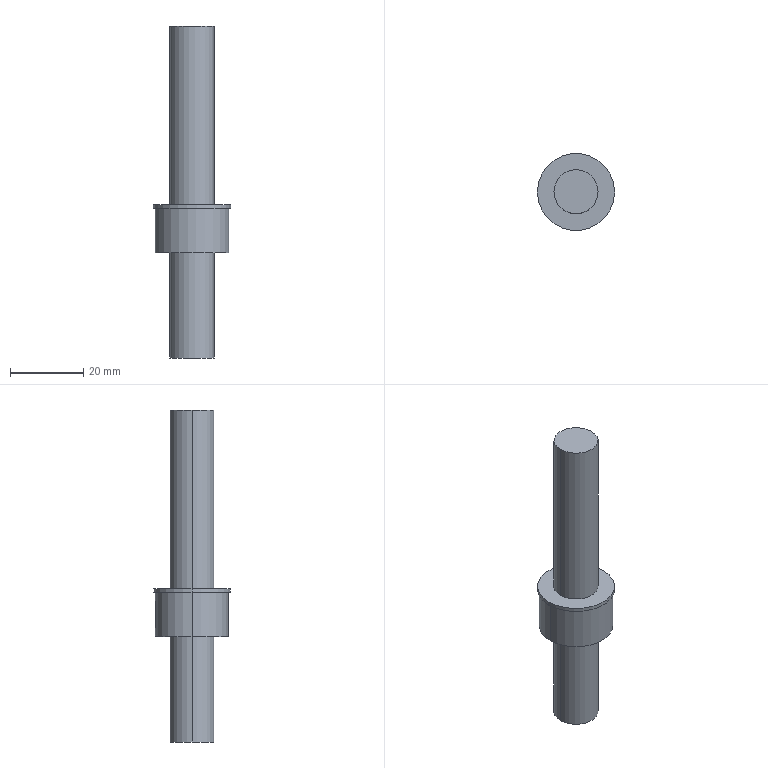Part | SolidWorks | features ICE 4, Extrusion 1 | 1 solid | 19 faces | box 21 x 21 x 90.35 mm | volume 12865 mm3 | cylinder 11 | plane 8 | commonest cylinder face diameters 12 x4 3 x3 20 x2 21 x2
STEP:
#1=CARTESIAN_POINT('',(0.,9.1,38.75));
#2=VERTEX_POINT('',#1);
#3=CARTESIAN_POINT('',(1.5,9.1,37.25));
#4=VERTEX_POINT('',#3);
#5=CARTESIAN_POINT('',(0.,9.1,37.25));
#6=DIRECTION('',(0.,1.,0.));
#7=DIRECTION('',(0.,0.,1.));
#8=AXIS2_PLACEMENT_3D('',#5,#6,#7);
#9=CIRCLE('',#8,1.5);
#10=EDGE_CURVE('',#2,#4,#9,.T.);
#11=ORIENTED_EDGE('',*,*,#10,.F.);
#12=CARTESIAN_POINT('',(0.,10.,38.75));
#13=VERTEX_POINT('',#12);
#14=CARTESIAN_POINT('',(0.,9.1,38.75));
#15=DIRECTION('',(0.,1.,0.));
#16=VECTOR('',#15,1000.);
#17=LINE('',#14,#16);
#18=EDGE_CURVE('',#2,#13,#17,.T.);
#19=ORIENTED_EDGE('',*,*,#18,.T.);
#20=CARTESIAN_POINT('',(1.5,9.887,37.25));
#21=VERTEX_POINT('',#20);
#22=CARTESIAN_POINT('',(1.5,9.887,37.25));
#23=CARTESIAN_POINT('',(1.5,9.887,37.349));
#24=CARTESIAN_POINT('',(1.49,9.888,37.447));
#25=CARTESIAN_POINT('',(1.452,9.894,37.639));
#26=CARTESIAN_POINT('',(1.423,9.898,37.734));
#27=CARTESIAN_POINT('',(1.348,9.909,37.916));
#28=CARTESIAN_POINT('',(1.302,9.915,38.002));
#29=CARTESIAN_POINT('',(1.193,9.929,38.165));
#30=CARTESIAN_POINT('',(1.129,9.936,38.242));
#31=CARTESIAN_POINT('',(0.922,9.958,38.449));
#32=CARTESIAN_POINT('',(0.7548,9.973,38.561));
#33=CARTESIAN_POINT('',(0.3937,9.994,38.711));
#34=CARTESIAN_POINT('',(0.196,10.,38.75));
#35=CARTESIAN_POINT('',(0.,10.,38.75));
#36=B_SPLINE_CURVE_WITH_KNOTS('',3,(#22,#23,#24,#25,#26,#27,#28,#29,#30,#31,#32,#33,#34,#35),.UNSPECIFIED.,.F.,.F.,(4,2,2,2,2,2,4),(0.,0.0002936,0.0005872,0.0008808,0.001174,0.001762,0.002349),.UNSPECIFIED.);
#37=EDGE_CURVE('',#21,#13,#36,.T.);
#38=ORIENTED_EDGE('',*,*,#37,.F.);
#39=CARTESIAN_POINT('',(1.5,9.1,37.25));
#40=DIRECTION('',(0.,1.,0.));
#41=VECTOR('',#40,1000.);
#42=LINE('',#39,#41);
#43=EDGE_CURVE('',#4,#21,#42,.T.);
#44=ORIENTED_EDGE('',*,*,#43,.F.);
#45=EDGE_LOOP('',(#11,#19,#38,#44));
#46=FACE_OUTER_BOUND('',#45,.T.);
#47=CARTESIAN_POINT('',(0.,9.1,37.25));
#48=DIRECTION('',(0.,1.,0.));
#49=DIRECTION('',(0.,0.,1.));
#50=AXIS2_PLACEMENT_3D('',#47,#48,#49);
#51=CYLINDRICAL_SURFACE('',#50,1.5);
#52=ADVANCED_FACE('',(#46),#51,.F.);
#53=CARTESIAN_POINT('',(6.,0.,90.35));
#54=VERTEX_POINT('',#53);
#55=CARTESIAN_POINT('',(-6.,0.,90.35));
#56=VERTEX_POINT('',#55);
#57=CARTESIAN_POINT('',(0.,0.,90.35));
#58=DIRECTION('',(0.,0.,1.));
#59=DIRECTION('',(1.,0.,0.));
#60=AXIS2_PLACEMENT_3D('',#57,#58,#59);
#61=CIRCLE('',#60,6.);
#62=EDGE_CURVE('',#54,#56,#61,.T.);
#63=ORIENTED_EDGE('',*,*,#62,.F.);
#64=CARTESIAN_POINT('',(6.,0.,41.75));
#65=VERTEX_POINT('',#64);
#66=CARTESIAN_POINT('',(6.,0.,90.35));
#67=DIRECTION('',(0.,0.,-1.));
#68=VECTOR('',#67,1000.);
#69=LINE('',#66,#68);
#70=EDGE_CURVE('',#54,#65,#69,.T.);
#71=ORIENTED_EDGE('',*,*,#70,.T.);
#72=CARTESIAN_POINT('',(-6.,0.,41.75));
#73=VERTEX_POINT('',#72);
#74=CARTESIAN_POINT('',(0.,0.,41.75));
#75=DIRECTION('',(0.,0.,1.));
#76=DIRECTION('',(1.,0.,0.));
#77=AXIS2_PLACEMENT_3D('',#74,#75,#76);
#78=CIRCLE('',#77,6.);
#79=EDGE_CURVE('',#65,#73,#78,.T.);
#80=ORIENTED_EDGE('',*,*,#79,.T.);
#81=CARTESIAN_POINT('',(-6.,0.,90.35));
#82=DIRECTION('',(0.,0.,-1.));
#83=VECTOR('',#82,1000.);
#84=LINE('',#81,#83);
#85=EDGE_CURVE('',#56,#73,#84,.T.);
#86=ORIENTED_EDGE('',*,*,#85,.F.);
#87=EDGE_LOOP('',(#63,#71,#80,#86));
#88=FACE_OUTER_BOUND('',#87,.T.);
#89=CARTESIAN_POINT('',(0.,0.,90.35));
#90=DIRECTION('',(0.,0.,-1.));
#91=DIRECTION('',(-1.,0.,0.));
#92=AXIS2_PLACEMENT_3D('',#89,#90,#91);
#93=CYLINDRICAL_SURFACE('',#92,6.);
#94=ADVANCED_FACE('',(#88),#93,.T.);
#95=CARTESIAN_POINT('',(10.5,0.,41.75));
#96=VERTEX_POINT('',#95);
#97=CARTESIAN_POINT('',(-10.5,0.,41.75));
#98=VERTEX_POINT('',#97);
#99=CARTESIAN_POINT('',(0.,0.,41.75));
#100=DIRECTION('',(0.,0.,1.));
#101=DIRECTION('',(1.,0.,0.));
#102=AXIS2_PLACEMENT_3D('',#99,#100,#101);
#103=CIRCLE('',#102,10.5);
#104=EDGE_CURVE('',#96,#98,#103,.T.);
#105=ORIENTED_EDGE('',*,*,#104,.F.);
#106=CARTESIAN_POINT('',(10.5,0.,40.75));
#107=VERTEX_POINT('',#106);
#108=CARTESIAN_POINT('',(10.5,0.,41.75));
#109=DIRECTION('',(0.,0.,-1.));
#110=VECTOR('',#109,1000.);
#111=LINE('',#108,#110);
#112=EDGE_CURVE('',#96,#107,#111,.T.);
#113=ORIENTED_EDGE('',*,*,#112,.T.);
#114=CARTESIAN_POINT('',(-10.5,0.,40.75));
#115=VERTEX_POINT('',#114);
#116=CARTESIAN_POINT('',(0.,0.,40.75));
#117=DIRECTION('',(0.,0.,1.));
#118=DIRECTION('',(1.,0.,0.));
#119=AXIS2_PLACEMENT_3D('',#116,#117,#118);
#120=CIRCLE('',#119,10.5);
#121=EDGE_CURVE('',#107,#115,#120,.T.);
#122=ORIENTED_EDGE('',*,*,#121,.T.);
#123=CARTESIAN_POINT('',(-10.5,0.,41.75));
#124=DIRECTION('',(0.,0.,-1.));
#125=VECTOR('',#124,1000.);
#126=LINE('',#123,#125);
#127=EDGE_CURVE('',#98,#115,#126,.T.);
#128=ORIENTED_EDGE('',*,*,#127,.F.);
#129=EDGE_LOOP('',(#105,#113,#122,#128));
#130=FACE_OUTER_BOUND('',#129,.T.);
#131=CARTESIAN_POINT('',(0.,0.,41.75));
#132=DIRECTION('',(0.,0.,-1.));
#133=DIRECTION('',(-1.,0.,0.));
#134=AXIS2_PLACEMENT_3D('',#131,#132,#133);
#135=CYLINDRICAL_SURFACE('',#134,10.5);
#136=ADVANCED_FACE('',(#130),#135,.T.);
#137=CARTESIAN_POINT('',(-1.5,9.887,37.25));
#138=VERTEX_POINT('',#137);
#139=CARTESIAN_POINT('',(-1.5,9.887,32.25));
#140=VERTEX_POINT('',#139);
#141=CARTESIAN_POINT('',(-1.5,9.887,40.75));
#142=DIRECTION('',(0.,0.,-1.));
#143=VECTOR('',#142,1000.);
#144=LINE('',#141,#143);
#145=EDGE_CURVE('',#138,#140,#144,.T.);
#146=ORIENTED_EDGE('',*,*,#145,.T.);
#147=CARTESIAN_POINT('',(1.5,9.887,32.25));
#148=VERTEX_POINT('',#147);
#149=CARTESIAN_POINT('',(-1.5,9.887,32.25));
#150=CARTESIAN_POINT('',(-1.5,9.887,32.151));
#151=CARTESIAN_POINT('',(-1.49,9.888,32.053));
#152=CARTESIAN_POINT('',(-1.452,9.894,31.861));
#153=CARTESIAN_POINT('',(-1.423,9.898,31.766));
#154=CARTESIAN_POINT('',(-1.348,9.909,31.584));
#155=CARTESIAN_POINT('',(-1.302,9.915,31.498));
#156=CARTESIAN_POINT('',(-1.193,9.929,31.335));
#157=CARTESIAN_POINT('',(-1.13,9.936,31.258));
#158=CARTESIAN_POINT('',(-0.9225,9.958,31.051));
#159=CARTESIAN_POINT('',(-0.7554,9.973,30.939));
#160=CARTESIAN_POINT('',(-0.3946,9.994,30.79));
#161=CARTESIAN_POINT('',(-0.1971,10.,30.75));
#162=CARTESIAN_POINT('',(0.09684,10.,30.75));
#163=CARTESIAN_POINT('',(0.1964,9.999,30.76));
#164=CARTESIAN_POINT('',(0.3888,9.993,30.798));
#165=CARTESIAN_POINT('',(0.4824,9.989,30.826));
#166=CARTESIAN_POINT('',(0.7551,9.973,30.939));
#167=CARTESIAN_POINT('',(0.9202,9.959,31.049));
#168=CARTESIAN_POINT('',(1.13,9.936,31.259));
#169=CARTESIAN_POINT('',(1.192,9.929,31.334));
#170=CARTESIAN_POINT('',(1.301,9.915,31.496));
#171=CARTESIAN_POINT('',(1.348,9.909,31.584));
#172=CARTESIAN_POINT('',(1.461,9.893,31.856));
#173=CARTESIAN_POINT('',(1.5,9.887,32.052));
#174=CARTESIAN_POINT('',(1.5,9.887,32.25));
#175=B_SPLINE_CURVE_WITH_KNOTS('',3,(#149,#150,#151,#152,#153,#154,#155,#156,#157,#158,#159,#160,#161,#162,#163,#164,#165,#166,#167,#168,#169,#170,#171,#172,#173,#174),.UNSPECIFIED.,.F.,.F.,(4,2,2,2,2,2,2,2,2,2,2,2,4),(0.,0.0002934,0.0005869,0.0008803,0.001174,0.001761,0.002348,0.002641,0.002934,0.003521,0.003815,0.004108,0.004695),.UNSPECIFIED.);
#176=EDGE_CURVE('',#140,#148,#175,.T.);
#177=ORIENTED_EDGE('',*,*,#176,.T.);
#178=CARTESIAN_POINT('',(1.5,9.887,40.75));
#179=DIRECTION('',(0.,0.,1.));
#180=VECTOR('',#179,1000.);
#181=LINE('',#178,#180);
#182=EDGE_CURVE('',#148,#21,#181,.T.);
#183=ORIENTED_EDGE('',*,*,#182,.T.);
#184=ORIENTED_EDGE('',*,*,#37,.T.);
#185=CARTESIAN_POINT('',(0.,10.,38.75));
#186=CARTESIAN_POINT('',(-0.09792,10.,38.75));
#187=CARTESIAN_POINT('',(-0.1974,9.999,38.74));
#188=CARTESIAN_POINT('',(-0.3897,9.993,38.702));
#189=CARTESIAN_POINT('',(-0.4832,9.989,38.673));
#190=CARTESIAN_POINT('',(-0.7557,9.973,38.561));
#191=CARTESIAN_POINT('',(-0.9207,9.959,38.451));
#192=CARTESIAN_POINT('',(-1.13,9.936,38.241));
#193=CARTESIAN_POINT('',(-1.192,9.929,38.166));
#194=CARTESIAN_POINT('',(-1.301,9.915,38.003));
#195=CARTESIAN_POINT('',(-1.348,9.909,37.916));
#196=CARTESIAN_POINT('',(-1.461,9.893,37.644));
#197=CARTESIAN_POINT('',(-1.5,9.887,37.448));
#198=CARTESIAN_POINT('',(-1.5,9.887,37.25));
#199=B_SPLINE_CURVE_WITH_KNOTS('',3,(#185,#186,#187,#188,#189,#190,#191,#192,#193,#194,#195,#196,#197,#198),.UNSPECIFIED.,.F.,.F.,(4,2,2,2,2,2,4),(0.002349,0.002642,0.002935,0.003522,0.003815,0.004109,0.004695),.UNSPECIFIED.);
#200=EDGE_CURVE('',#13,#138,#199,.T.);
#201=ORIENTED_EDGE('',*,*,#200,.T.);
#202=EDGE_LOOP('',(#146,#177,#183,#184,#201));
#203=FACE_BOUND('',#202,.T.);
#204=CARTESIAN_POINT('',(10.,0.,40.75));
#205=VERTEX_POINT('',#204);
#206=CARTESIAN_POINT('',(-10.,0.,40.75));
#207=VERTEX_POINT('',#206);
#208=CARTESIAN_POINT('',(0.,0.,40.75));
#209=DIRECTION('',(0.,0.,1.));
#210=DIRECTION('',(1.,0.,0.));
#211=AXIS2_PLACEMENT_3D('',#208,#209,#210);
#212=CIRCLE('',#211,10.);
#213=EDGE_CURVE('',#205,#207,#212,.T.);
#214=ORIENTED_EDGE('',*,*,#213,.F.);
#215=CARTESIAN_POINT('',(10.,0.,28.65));
#216=VERTEX_POINT('',#215);
#217=CARTESIAN_POINT('',(10.,0.,40.75));
#218=DIRECTION('',(0.,0.,-1.));
#219=VECTOR('',#218,1000.);
#220=LINE('',#217,#219);
#221=EDGE_CURVE('',#205,#216,#220,.T.);
#222=ORIENTED_EDGE('',*,*,#221,.T.);
#223=CARTESIAN_POINT('',(-10.,0.,28.65));
#224=VERTEX_POINT('',#223);
#225=CARTESIAN_POINT('',(0.,0.,28.65));
#226=DIRECTION('',(0.,0.,1.));
#227=DIRECTION('',(1.,0.,0.));
#228=AXIS2_PLACEMENT_3D('',#225,#226,#227);
#229=CIRCLE('',#228,10.);
#230=EDGE_CURVE('',#216,#224,#229,.T.);
#231=ORIENTED_EDGE('',*,*,#230,.T.);
#232=CARTESIAN_POINT('',(-10.,0.,40.75));
#233=DIRECTION('',(0.,0.,-1.));
#234=VECTOR('',#233,1000.);
#235=LINE('',#232,#234);
#236=EDGE_CURVE('',#207,#224,#235,.T.);
#237=ORIENTED_EDGE('',*,*,#236,.F.);
#238=EDGE_LOOP('',(#214,#222,#231,#237));
#239=FACE_OUTER_BOUND('',#238,.T.);
#240=CARTESIAN_POINT('',(0.,0.,40.75));
#241=DIRECTION('',(0.,0.,-1.));
#242=DIRECTION('',(-1.,0.,0.));
#243=AXIS2_PLACEMENT_3D('',#240,#241,#242);
#244=CYLINDRICAL_SURFACE('',#243,10.);
#245=ADVANCED_FACE('',(#203,#239),#244,.T.);
#246=CARTESIAN_POINT('',(6.,0.,28.65));
#247=VERTEX_POINT('',#246);
#248=CARTESIAN_POINT('',(-6.,0.,28.65));
#249=VERTEX_POINT('',#248);
#250=CARTESIAN_POINT('',(0.,0.,28.65));
#251=DIRECTION('',(0.,0.,1.));
#252=DIRECTION('',(1.,0.,0.));
#253=AXIS2_PLACEMENT_3D('',#250,#251,#252);
#254=CIRCLE('',#253,6.);
#255=EDGE_CURVE('',#247,#249,#254,.T.);
#256=ORIENTED_EDGE('',*,*,#255,.F.);
#257=CARTESIAN_POINT('',(6.,0.,0.));
#258=VERTEX_POINT('',#257);
#259=CARTESIAN_POINT('',(6.,0.,28.65));
#260=DIRECTION('',(0.,0.,-1.));
#261=VECTOR('',#260,1000.);
#262=LINE('',#259,#261);
#263=EDGE_CURVE('',#247,#258,#262,.T.);
#264=ORIENTED_EDGE('',*,*,#263,.T.);
#265=CARTESIAN_POINT('',(-6.,0.,0.));
#266=VERTEX_POINT('',#265);
#267=CARTESIAN_POINT('',(0.,0.,0.));
#268=DIRECTION('',(0.,0.,1.));
#269=DIRECTION('',(1.,0.,0.));
#270=AXIS2_PLACEMENT_3D('',#267,#268,#269);
#271=CIRCLE('',#270,6.);
#272=EDGE_CURVE('',#258,#266,#271,.T.);
#273=ORIENTED_EDGE('',*,*,#272,.T.);
#274=CARTESIAN_POINT('',(-6.,0.,28.65));
#275=DIRECTION('',(0.,0.,-1.));
#276=VECTOR('',#275,1000.);
#277=LINE('',#274,#276);
#278=EDGE_CURVE('',#249,#266,#277,.T.);
#279=ORIENTED_EDGE('',*,*,#278,.F.);
#280=EDGE_LOOP('',(#256,#264,#273,#279));
#281=FACE_OUTER_BOUND('',#280,.T.);
#282=CARTESIAN_POINT('',(0.,0.,28.65));
#283=DIRECTION('',(0.,0.,-1.));
#284=DIRECTION('',(-1.,0.,0.));
#285=AXIS2_PLACEMENT_3D('',#282,#283,#284);
#286=CYLINDRICAL_SURFACE('',#285,6.);
#287=ADVANCED_FACE('',(#281),#286,.T.);
#288=ORIENTED_EDGE('',*,*,#263,.F.);
#289=CARTESIAN_POINT('',(0.,0.,28.65));
#290=DIRECTION('',(0.,0.,1.));
#291=DIRECTION('',(1.,0.,0.));
#292=AXIS2_PLACEMENT_3D('',#289,#290,#291);
#293=CIRCLE('',#292,6.);
#294=EDGE_CURVE('',#249,#247,#293,.T.);
#295=ORIENTED_EDGE('',*,*,#294,.F.);
#296=ORIENTED_EDGE('',*,*,#278,.T.);
#297=CARTESIAN_POINT('',(0.,0.,0.));
#298=DIRECTION('',(0.,0.,1.));
#299=DIRECTION('',(1.,0.,0.));
#300=AXIS2_PLACEMENT_3D('',#297,#298,#299);
#301=CIRCLE('',#300,6.);
#302=EDGE_CURVE('',#266,#258,#301,.T.);
#303=ORIENTED_EDGE('',*,*,#302,.T.);
#304=EDGE_LOOP('',(#288,#295,#296,#303));
#305=FACE_OUTER_BOUND('',#304,.T.);
#306=CARTESIAN_POINT('',(0.,0.,28.65));
#307=DIRECTION('',(0.,0.,-1.));
#308=DIRECTION('',(-1.,0.,0.));
#309=AXIS2_PLACEMENT_3D('',#306,#307,#308);
#310=CYLINDRICAL_SURFACE('',#309,6.);
#311=ADVANCED_FACE('',(#305),#310,.T.);
#312=ORIENTED_EDGE('',*,*,#302,.F.);
#313=ORIENTED_EDGE('',*,*,#272,.F.);
#314=EDGE_LOOP('',(#312,#313));
#315=FACE_OUTER_BOUND('',#314,.T.);
#316=CARTESIAN_POINT('',(0.,0.,0.));
#317=DIRECTION('',(0.,0.,1.));
#318=DIRECTION('',(1.,0.,0.));
#319=AXIS2_PLACEMENT_3D('',#316,#317,#318);
#320=PLANE('',#319);
#321=ADVANCED_FACE('',(#315),#320,.F.);
#322=ORIENTED_EDGE('',*,*,#221,.F.);
#323=CARTESIAN_POINT('',(0.,0.,40.75));
#324=DIRECTION('',(0.,0.,1.));
#325=DIRECTION('',(1.,0.,0.));
#326=AXIS2_PLACEMENT_3D('',#323,#324,#325);
#327=CIRCLE('',#326,10.);
#328=EDGE_CURVE('',#207,#205,#327,.T.);
#329=ORIENTED_EDGE('',*,*,#328,.F.);
#330=ORIENTED_EDGE('',*,*,#236,.T.);
#331=CARTESIAN_POINT('',(0.,0.,28.65));
#332=DIRECTION('',(0.,0.,1.));
#333=DIRECTION('',(1.,0.,0.));
#334=AXIS2_PLACEMENT_3D('',#331,#332,#333);
#335=CIRCLE('',#334,10.);
#336=EDGE_CURVE('',#224,#216,#335,.T.);
#337=ORIENTED_EDGE('',*,*,#336,.T.);
#338=EDGE_LOOP('',(#322,#329,#330,#337));
#339=FACE_OUTER_BOUND('',#338,.T.);
#340=CARTESIAN_POINT('',(0.,0.,40.75));
#341=DIRECTION('',(0.,0.,-1.));
#342=DIRECTION('',(-1.,0.,0.));
#343=AXIS2_PLACEMENT_3D('',#340,#341,#342);
#344=CYLINDRICAL_SURFACE('',#343,10.);
#345=ADVANCED_FACE('',(#339),#344,.T.);
#346=ORIENTED_EDGE('',*,*,#294,.T.);
#347=ORIENTED_EDGE('',*,*,#255,.T.);
#348=EDGE_LOOP('',(#346,#347));
#349=FACE_BOUND('',#348,.T.);
#350=ORIENTED_EDGE('',*,*,#336,.F.);
#351=ORIENTED_EDGE('',*,*,#230,.F.);
#352=EDGE_LOOP('',(#350,#351));
#353=FACE_OUTER_BOUND('',#352,.T.);
#354=CARTESIAN_POINT('',(0.,0.,28.65));
#355=DIRECTION('',(0.,0.,1.));
#356=DIRECTION('',(1.,0.,0.));
#357=AXIS2_PLACEMENT_3D('',#354,#355,#356);
#358=PLANE('',#357);
#359=ADVANCED_FACE('',(#349,#353),#358,.F.);
#360=ORIENTED_EDGE('',*,*,#112,.F.);
#361=CARTESIAN_POINT('',(0.,0.,41.75));
#362=DIRECTION('',(0.,0.,1.));
#363=DIRECTION('',(1.,0.,0.));
#364=AXIS2_PLACEMENT_3D('',#361,#362,#363);
#365=CIRCLE('',#364,10.5);
#366=EDGE_CURVE('',#98,#96,#365,.T.);
#367=ORIENTED_EDGE('',*,*,#366,.F.);
#368=ORIENTED_EDGE('',*,*,#127,.T.);
#369=CARTESIAN_POINT('',(0.,0.,40.75));
#370=DIRECTION('',(0.,0.,1.));
#371=DIRECTION('',(1.,0.,0.));
#372=AXIS2_PLACEMENT_3D('',#369,#370,#371);
#373=CIRCLE('',#372,10.5);
#374=EDGE_CURVE('',#115,#107,#373,.T.);
#375=ORIENTED_EDGE('',*,*,#374,.T.);
#376=EDGE_LOOP('',(#360,#367,#368,#375));
#377=FACE_OUTER_BOUND('',#376,.T.);
#378=CARTESIAN_POINT('',(0.,0.,41.75));
#379=DIRECTION('',(0.,0.,-1.));
#380=DIRECTION('',(-1.,0.,0.));
#381=AXIS2_PLACEMENT_3D('',#378,#379,#380);
#382=CYLINDRICAL_SURFACE('',#381,10.5);
#383=ADVANCED_FACE('',(#377),#382,.T.);
#384=CARTESIAN_POINT('',(0.,0.,41.75));
#385=DIRECTION('',(0.,0.,1.));
#386=DIRECTION('',(1.,0.,0.));
#387=AXIS2_PLACEMENT_3D('',#384,#385,#386);
#388=CIRCLE('',#387,6.);
#389=EDGE_CURVE('',#73,#65,#388,.T.);
#390=ORIENTED_EDGE('',*,*,#389,.F.);
#391=ORIENTED_EDGE('',*,*,#79,.F.);
#392=EDGE_LOOP('',(#390,#391));
#393=FACE_BOUND('',#392,.T.);
#394=ORIENTED_EDGE('',*,*,#366,.T.);
#395=ORIENTED_EDGE('',*,*,#104,.T.);
#396=EDGE_LOOP('',(#394,#395));
#397=FACE_OUTER_BOUND('',#396,.T.);
#398=CARTESIAN_POINT('',(0.,0.,41.75));
#399=DIRECTION('',(0.,0.,1.));
#400=DIRECTION('',(1.,0.,0.));
#401=AXIS2_PLACEMENT_3D('',#398,#399,#400);
#402=PLANE('',#401);
#403=ADVANCED_FACE('',(#393,#397),#402,.T.);
#404=ORIENTED_EDGE('',*,*,#328,.T.);
#405=ORIENTED_EDGE('',*,*,#213,.T.);
#406=EDGE_LOOP('',(#404,#405));
#407=FACE_BOUND('',#406,.T.);
#408=ORIENTED_EDGE('',*,*,#374,.F.);
#409=ORIENTED_EDGE('',*,*,#121,.F.);
#410=EDGE_LOOP('',(#408,#409));
#411=FACE_OUTER_BOUND('',#410,.T.);
#412=CARTESIAN_POINT('',(0.,0.,40.75));
#413=DIRECTION('',(0.,0.,1.));
#414=DIRECTION('',(1.,0.,0.));
#415=AXIS2_PLACEMENT_3D('',#412,#413,#414);
#416=PLANE('',#415);
#417=ADVANCED_FACE('',(#407,#411),#416,.F.);
#418=ORIENTED_EDGE('',*,*,#70,.F.);
#419=CARTESIAN_POINT('',(0.,0.,90.35));
#420=DIRECTION('',(0.,0.,1.));
#421=DIRECTION('',(1.,0.,0.));
#422=AXIS2_PLACEMENT_3D('',#419,#420,#421);
#423=CIRCLE('',#422,6.);
#424=EDGE_CURVE('',#56,#54,#423,.T.);
#425=ORIENTED_EDGE('',*,*,#424,.F.);
#426=ORIENTED_EDGE('',*,*,#85,.T.);
#427=ORIENTED_EDGE('',*,*,#389,.T.);
#428=EDGE_LOOP('',(#418,#425,#426,#427));
#429=FACE_OUTER_BOUND('',#428,.T.);
#430=CARTESIAN_POINT('',(0.,0.,90.35));
#431=DIRECTION('',(0.,0.,-1.));
#432=DIRECTION('',(-1.,0.,0.));
#433=AXIS2_PLACEMENT_3D('',#430,#431,#432);
#434=CYLINDRICAL_SURFACE('',#433,6.);
#435=ADVANCED_FACE('',(#429),#434,.T.);
#436=ORIENTED_EDGE('',*,*,#424,.T.);
#437=ORIENTED_EDGE('',*,*,#62,.T.);
#438=EDGE_LOOP('',(#436,#437));
#439=FACE_OUTER_BOUND('',#438,.T.);
#440=CARTESIAN_POINT('',(0.,0.,90.35));
#441=DIRECTION('',(0.,0.,1.));
#442=DIRECTION('',(1.,0.,0.));
#443=AXIS2_PLACEMENT_3D('',#440,#441,#442);
#444=PLANE('',#443);
#445=ADVANCED_FACE('',(#439),#444,.T.);
#446=CARTESIAN_POINT('',(-1.5,9.1,32.25));
#447=VERTEX_POINT('',#446);
#448=CARTESIAN_POINT('',(-1.5,9.1,32.25));
#449=DIRECTION('',(0.,1.,0.));
#450=VECTOR('',#449,1000.);
#451=LINE('',#448,#450);
#452=EDGE_CURVE('',#447,#140,#451,.T.);
#453=ORIENTED_EDGE('',*,*,#452,.F.);
#454=CARTESIAN_POINT('',(1.5,9.1,32.25));
#455=VERTEX_POINT('',#454);
#456=CARTESIAN_POINT('',(0.,9.1,32.25));
#457=DIRECTION('',(0.,1.,0.));
#458=DIRECTION('',(0.,0.,1.));
#459=AXIS2_PLACEMENT_3D('',#456,#457,#458);
#460=CIRCLE('',#459,1.5);
#461=EDGE_CURVE('',#455,#447,#460,.T.);
#462=ORIENTED_EDGE('',*,*,#461,.F.);
#463=CARTESIAN_POINT('',(1.5,9.1,32.25));
#464=DIRECTION('',(0.,1.,0.));
#465=VECTOR('',#464,1000.);
#466=LINE('',#463,#465);
#467=EDGE_CURVE('',#455,#148,#466,.T.);
#468=ORIENTED_EDGE('',*,*,#467,.T.);
#469=ORIENTED_EDGE('',*,*,#176,.F.);
#470=EDGE_LOOP('',(#453,#462,#468,#469));
#471=FACE_OUTER_BOUND('',#470,.T.);
#472=CARTESIAN_POINT('',(0.,9.1,32.25));
#473=DIRECTION('',(0.,1.,0.));
#474=DIRECTION('',(0.,0.,1.));
#475=AXIS2_PLACEMENT_3D('',#472,#473,#474);
#476=CYLINDRICAL_SURFACE('',#475,1.5);
#477=ADVANCED_FACE('',(#471),#476,.F.);
#478=ORIENTED_EDGE('',*,*,#467,.F.);
#479=CARTESIAN_POINT('',(1.5,9.1,32.25));
#480=DIRECTION('',(0.,0.,-1.));
#481=VECTOR('',#480,1000.);
#482=LINE('',#479,#481);
#483=EDGE_CURVE('',#4,#455,#482,.T.);
#484=ORIENTED_EDGE('',*,*,#483,.F.);
#485=ORIENTED_EDGE('',*,*,#43,.T.);
#486=ORIENTED_EDGE('',*,*,#182,.F.);
#487=EDGE_LOOP('',(#478,#484,#485,#486));
#488=FACE_OUTER_BOUND('',#487,.T.);
#489=CARTESIAN_POINT('',(1.5,9.1,32.25));
#490=DIRECTION('',(1.,0.,0.));
#491=DIRECTION('',(0.,0.,-1.));
#492=AXIS2_PLACEMENT_3D('',#489,#490,#491);
#493=PLANE('',#492);
#494=ADVANCED_FACE('',(#488),#493,.F.);
#495=ORIENTED_EDGE('',*,*,#18,.F.);
#496=CARTESIAN_POINT('',(-1.5,9.1,37.25));
#497=VERTEX_POINT('',#496);
#498=CARTESIAN_POINT('',(0.,9.1,37.25));
#499=DIRECTION('',(0.,1.,0.));
#500=DIRECTION('',(0.,0.,1.));
#501=AXIS2_PLACEMENT_3D('',#498,#499,#500);
#502=CIRCLE('',#501,1.5);
#503=EDGE_CURVE('',#497,#2,#502,.T.);
#504=ORIENTED_EDGE('',*,*,#503,.F.);
#505=CARTESIAN_POINT('',(-1.5,9.1,37.25));
#506=DIRECTION('',(0.,1.,0.));
#507=VECTOR('',#506,1000.);
#508=LINE('',#505,#507);
#509=EDGE_CURVE('',#497,#138,#508,.T.);
#510=ORIENTED_EDGE('',*,*,#509,.T.);
#511=ORIENTED_EDGE('',*,*,#200,.F.);
#512=EDGE_LOOP('',(#495,#504,#510,#511));
#513=FACE_OUTER_BOUND('',#512,.T.);
#514=CARTESIAN_POINT('',(0.,9.1,37.25));
#515=DIRECTION('',(0.,1.,0.));
#516=DIRECTION('',(0.,0.,1.));
#517=AXIS2_PLACEMENT_3D('',#514,#515,#516);
#518=CYLINDRICAL_SURFACE('',#517,1.5);
#519=ADVANCED_FACE('',(#513),#518,.F.);
#520=ORIENTED_EDGE('',*,*,#509,.F.);
#521=CARTESIAN_POINT('',(-1.5,9.1,32.25));
#522=DIRECTION('',(0.,0.,1.));
#523=VECTOR('',#522,1000.);
#524=LINE('',#521,#523);
#525=EDGE_CURVE('',#447,#497,#524,.T.);
#526=ORIENTED_EDGE('',*,*,#525,.F.);
#527=ORIENTED_EDGE('',*,*,#452,.T.);
#528=ORIENTED_EDGE('',*,*,#145,.F.);
#529=EDGE_LOOP('',(#520,#526,#527,#528));
#530=FACE_OUTER_BOUND('',#529,.T.);
#531=CARTESIAN_POINT('',(-1.5,9.1,32.25));
#532=DIRECTION('',(-1.,0.,0.));
#533=DIRECTION('',(0.,0.,1.));
#534=AXIS2_PLACEMENT_3D('',#531,#532,#533);
#535=PLANE('',#534);
#536=ADVANCED_FACE('',(#530),#535,.F.);
#537=ORIENTED_EDGE('',*,*,#461,.T.);
#538=ORIENTED_EDGE('',*,*,#525,.T.);
#539=ORIENTED_EDGE('',*,*,#503,.T.);
#540=ORIENTED_EDGE('',*,*,#10,.T.);
#541=ORIENTED_EDGE('',*,*,#483,.T.);
#542=EDGE_LOOP('',(#537,#538,#539,#540,#541));
#543=FACE_OUTER_BOUND('',#542,.T.);
#544=CARTESIAN_POINT('',(0.,9.1,32.25));
#545=DIRECTION('',(0.,1.,0.));
#546=DIRECTION('',(0.,0.,1.));
#547=AXIS2_PLACEMENT_3D('',#544,#545,#546);
#548=PLANE('',#547);
#549=ADVANCED_FACE('',(#543),#548,.T.);
#550=CLOSED_SHELL('',(#52,#94,#136,#245,#287,#311,#321,#345,#359,#383,#403,#417,#435,#445,#477,#494,#519,#536,#549));
#551=MANIFOLD_SOLID_BREP('',#550);
#552=CARTESIAN_POINT('',(0.,0.,0.));
#553=DIRECTION('',(0.,0.,1.));
#554=DIRECTION('',(1.,0.,0.));
#555=AXIS2_PLACEMENT_3D('',#552,#553,#554);
#556=(LENGTH_UNIT()NAMED_UNIT(*)SI_UNIT(.MILLI.,.METRE.));
#557=UNCERTAINTY_MEASURE_WITH_UNIT(LENGTH_MEASURE(0.00001),#556,'','');
#558=(NAMED_UNIT(*)PLANE_ANGLE_UNIT()SI_UNIT($,.RADIAN.));
#559=(NAMED_UNIT(*)SI_UNIT($,.STERADIAN.)SOLID_ANGLE_UNIT());
#560=(GEOMETRIC_REPRESENTATION_CONTEXT(3)GLOBAL_UNCERTAINTY_ASSIGNED_CONTEXT((#557))GLOBAL_UNIT_ASSIGNED_CONTEXT((#556,#558,#559))REPRESENTATION_CONTEXT('',''));
#561=ADVANCED_BREP_SHAPE_REPRESENTATION('',(#551,#555),#560);